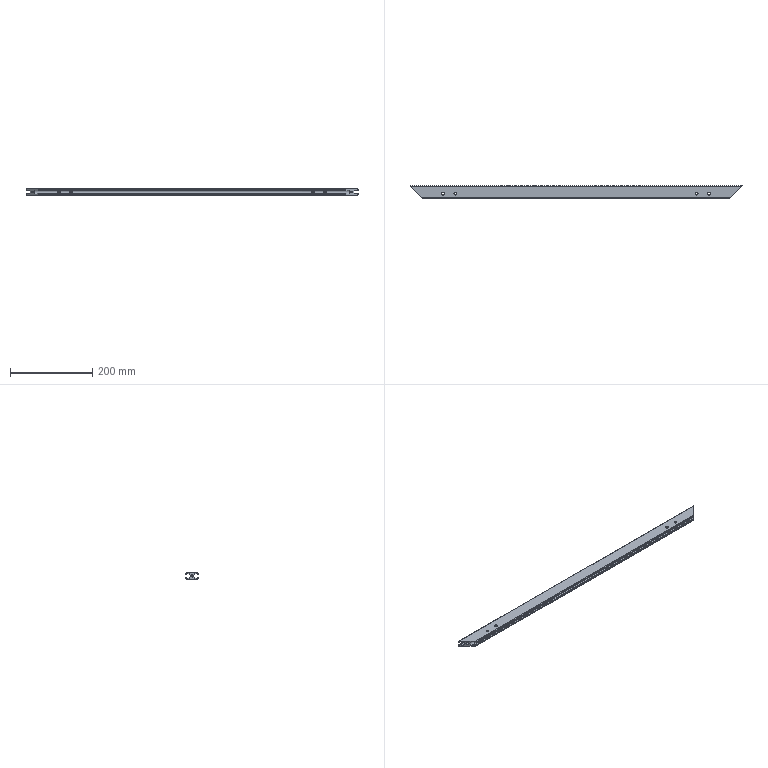Part | SolidWorks | features 3DProfileFeature 1, HoleWzd 1, ICE 1, WeldMemberFeat 1, WeldmentFeature 1 | 1 solid | 40 faces | box 805 x 30 x 15 mm | volume 189619 mm3 | cylinder 20 | plane 20 | commonest cylinder face diameters 6.8 x8 12 x6 3 x4 5 x2